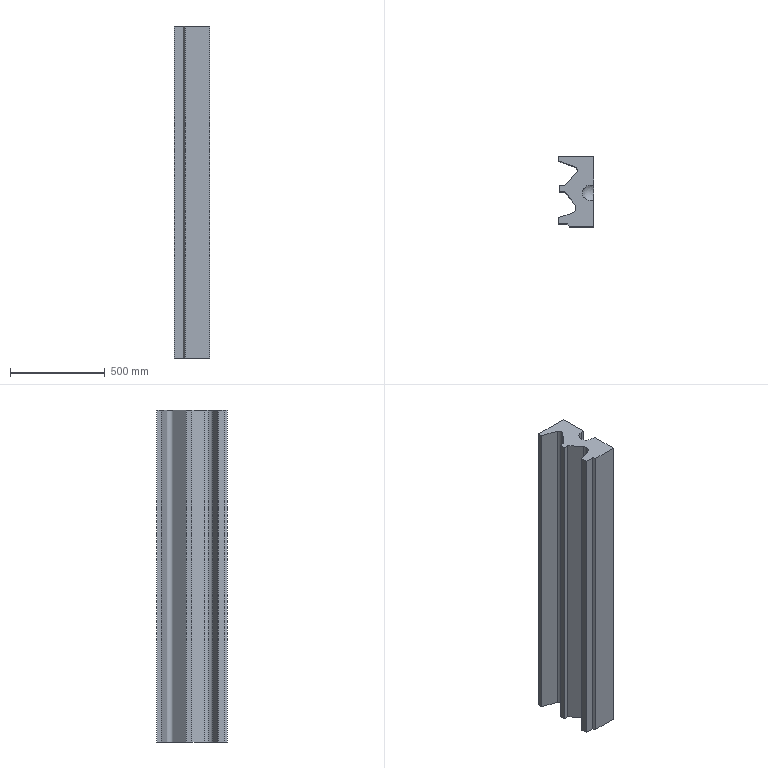Part | SolidWorks | features 3DProfileFeature 1, Extrusion 1, ICE 1, MirrorPattern 1, RevCut 1 | 1 solid | 33 faces | box 187.997 x 370.453 x 1750 mm | volume 86925596 mm3 | plane 24 | cylinder 5 | spline 2 | sphere 2 | commonest cylinder face diameters 80 x3 63.152 x2
STEP:
#1=CARTESIAN_POINT('',(-20.,75.362,-1650.));
#2=VERTEX_POINT('',#1);
#3=CARTESIAN_POINT('',(-60.,35.362,-1650.));
#4=VERTEX_POINT('',#3);
#5=CARTESIAN_POINT('',(-20.,35.362,-1650.));
#6=DIRECTION('',(0.,0.,1.));
#7=DIRECTION('',(-1.,0.,0.));
#8=AXIS2_PLACEMENT_3D('',#5,#6,#7);
#9=CIRCLE('',#8,40.);
#10=EDGE_CURVE('',#2,#4,#9,.T.);
#11=ORIENTED_EDGE('',*,*,#10,.T.);
#12=CARTESIAN_POINT('',(-60.,35.362,-1750.));
#13=VERTEX_POINT('',#12);
#14=CARTESIAN_POINT('',(-60.,35.362,-1650.));
#15=DIRECTION('',(0.,0.,-1.));
#16=VECTOR('',#15,1000.);
#17=LINE('',#14,#16);
#18=EDGE_CURVE('',#4,#13,#17,.T.);
#19=ORIENTED_EDGE('',*,*,#18,.T.);
#20=CARTESIAN_POINT('',(-20.,75.362,-1750.));
#21=VERTEX_POINT('',#20);
#22=CARTESIAN_POINT('',(-20.,35.362,-1750.));
#23=DIRECTION('',(0.,0.,1.));
#24=DIRECTION('',(-1.,0.,0.));
#25=AXIS2_PLACEMENT_3D('',#22,#23,#24);
#26=CIRCLE('',#25,40.);
#27=EDGE_CURVE('',#21,#13,#26,.T.);
#28=ORIENTED_EDGE('',*,*,#27,.F.);
#29=CARTESIAN_POINT('',(-20.,75.362,-1650.));
#30=DIRECTION('',(0.,0.,-1.));
#31=VECTOR('',#30,1000.);
#32=LINE('',#29,#31);
#33=EDGE_CURVE('',#2,#21,#32,.T.);
#34=ORIENTED_EDGE('',*,*,#33,.F.);
#35=EDGE_LOOP('',(#11,#19,#28,#34));
#36=FACE_OUTER_BOUND('',#35,.T.);
#37=CARTESIAN_POINT('',(-20.,35.362,-1650.));
#38=DIRECTION('',(0.,0.,-1.));
#39=DIRECTION('',(-1.,0.,0.));
#40=AXIS2_PLACEMENT_3D('',#37,#38,#39);
#41=CYLINDRICAL_SURFACE('',#40,40.);
#42=ADVANCED_FACE('',(#36),#41,.F.);
#43=CARTESIAN_POINT('',(-95.739,-44.185,-1750.));
#44=VERTEX_POINT('',#43);
#45=CARTESIAN_POINT('',(-102.315,-24.897,-1750.));
#46=VERTEX_POINT('',#45);
#47=CARTESIAN_POINT('',(-127.315,-44.185,-1750.));
#48=DIRECTION('',(0.,0.,1.));
#49=DIRECTION('',(1.,0.,0.));
#50=AXIS2_PLACEMENT_3D('',#47,#48,#49);
#51=CIRCLE('',#50,31.576);
#52=EDGE_CURVE('',#44,#46,#51,.T.);
#53=ORIENTED_EDGE('',*,*,#52,.F.);
#54=CARTESIAN_POINT('',(-95.739,-44.185,0.));
#55=VERTEX_POINT('',#54);
#56=CARTESIAN_POINT('',(-95.739,-44.185,-1750.));
#57=DIRECTION('',(0.,0.,1.));
#58=VECTOR('',#57,1000.);
#59=LINE('',#56,#58);
#60=EDGE_CURVE('',#44,#55,#59,.T.);
#61=ORIENTED_EDGE('',*,*,#60,.T.);
#62=CARTESIAN_POINT('',(-102.315,-24.897,0.));
#63=VERTEX_POINT('',#62);
#64=CARTESIAN_POINT('',(-127.315,-44.185,0.));
#65=DIRECTION('',(0.,0.,1.));
#66=DIRECTION('',(1.,0.,0.));
#67=AXIS2_PLACEMENT_3D('',#64,#65,#66);
#68=CIRCLE('',#67,31.576);
#69=EDGE_CURVE('',#55,#63,#68,.T.);
#70=ORIENTED_EDGE('',*,*,#69,.T.);
#71=CARTESIAN_POINT('',(-102.315,-24.897,-1750.));
#72=DIRECTION('',(0.,0.,1.));
#73=VECTOR('',#72,1000.);
#74=LINE('',#71,#73);
#75=EDGE_CURVE('',#46,#63,#74,.T.);
#76=ORIENTED_EDGE('',*,*,#75,.F.);
#77=EDGE_LOOP('',(#53,#61,#70,#76));
#78=FACE_OUTER_BOUND('',#77,.T.);
#79=CARTESIAN_POINT('',(-127.315,-44.185,-1750.));
#80=DIRECTION('',(0.,0.,1.));
#81=DIRECTION('',(1.,0.,0.));
#82=AXIS2_PLACEMENT_3D('',#79,#80,#81);
#83=CYLINDRICAL_SURFACE('',#82,31.576);
#84=ADVANCED_FACE('',(#78),#83,.F.);
#85=CARTESIAN_POINT('',(0.,-4.638,-1650.));
#86=VERTEX_POINT('',#85);
#87=CARTESIAN_POINT('',(0.,-24.638,-1650.));
#88=VERTEX_POINT('',#87);
#89=CARTESIAN_POINT('',(0.,95.362,-1650.));
#90=DIRECTION('',(0.,-1.,0.));
#91=VECTOR('',#90,1000.);
#92=LINE('',#89,#91);
#93=EDGE_CURVE('',#86,#88,#92,.T.);
#94=ORIENTED_EDGE('',*,*,#93,.T.);
#95=CARTESIAN_POINT('',(0.,95.362,-1650.));
#96=VERTEX_POINT('',#95);
#97=CARTESIAN_POINT('',(0.,35.362,-1650.));
#98=DIRECTION('',(-1.,0.,0.));
#99=DIRECTION('',(0.,-1.,0.));
#100=AXIS2_PLACEMENT_3D('',#97,#98,#99);
#101=CIRCLE('',#100,60.);
#102=EDGE_CURVE('',#88,#96,#101,.T.);
#103=ORIENTED_EDGE('',*,*,#102,.T.);
#104=CARTESIAN_POINT('',(0.,75.362,-1650.));
#105=VERTEX_POINT('',#104);
#106=CARTESIAN_POINT('',(0.,95.362,-1650.));
#107=DIRECTION('',(0.,-1.,0.));
#108=VECTOR('',#107,1000.);
#109=LINE('',#106,#108);
#110=EDGE_CURVE('',#96,#105,#109,.T.);
#111=ORIENTED_EDGE('',*,*,#110,.T.);
#112=CARTESIAN_POINT('',(0.,75.362,-1750.));
#113=VERTEX_POINT('',#112);
#114=CARTESIAN_POINT('',(0.,75.362,-1650.));
#115=DIRECTION('',(0.,0.,-1.));
#116=VECTOR('',#115,1000.);
#117=LINE('',#114,#116);
#118=EDGE_CURVE('',#105,#113,#117,.T.);
#119=ORIENTED_EDGE('',*,*,#118,.T.);
#120=CARTESIAN_POINT('',(0.,225.815,-1750.));
#121=VERTEX_POINT('',#120);
#122=CARTESIAN_POINT('',(0.,0.,-1750.));
#123=DIRECTION('',(0.,1.,0.));
#124=VECTOR('',#123,1000.);
#125=LINE('',#122,#124);
#126=EDGE_CURVE('',#113,#121,#125,.T.);
#127=ORIENTED_EDGE('',*,*,#126,.T.);
#128=CARTESIAN_POINT('',(0.,225.815,0.));
#129=VERTEX_POINT('',#128);
#130=CARTESIAN_POINT('',(0.,225.815,-1750.));
#131=DIRECTION('',(0.,0.,1.));
#132=VECTOR('',#131,1000.);
#133=LINE('',#130,#132);
#134=EDGE_CURVE('',#121,#129,#133,.T.);
#135=ORIENTED_EDGE('',*,*,#134,.T.);
#136=CARTESIAN_POINT('',(0.,75.362,0.));
#137=VERTEX_POINT('',#136);
#138=CARTESIAN_POINT('',(0.,0.,0.));
#139=DIRECTION('',(0.,1.,0.));
#140=VECTOR('',#139,1000.);
#141=LINE('',#138,#140);
#142=EDGE_CURVE('',#137,#129,#141,.T.);
#143=ORIENTED_EDGE('',*,*,#142,.F.);
#144=CARTESIAN_POINT('',(0.,75.362,-100.));
#145=VERTEX_POINT('',#144);
#146=CARTESIAN_POINT('',(0.,75.362,-100.));
#147=DIRECTION('',(0.,0.,1.));
#148=VECTOR('',#147,1000.);
#149=LINE('',#146,#148);
#150=EDGE_CURVE('',#145,#137,#149,.T.);
#151=ORIENTED_EDGE('',*,*,#150,.F.);
#152=CARTESIAN_POINT('',(0.,95.362,-100.));
#153=VERTEX_POINT('',#152);
#154=CARTESIAN_POINT('',(0.,95.362,-100.));
#155=DIRECTION('',(0.,-1.,0.));
#156=VECTOR('',#155,1000.);
#157=LINE('',#154,#156);
#158=EDGE_CURVE('',#153,#145,#157,.T.);
#159=ORIENTED_EDGE('',*,*,#158,.F.);
#160=CARTESIAN_POINT('',(0.,-24.638,-100.));
#161=VERTEX_POINT('',#160);
#162=CARTESIAN_POINT('',(0.,35.362,-100.));
#163=DIRECTION('',(1.,0.,0.));
#164=DIRECTION('',(0.,-1.,0.));
#165=AXIS2_PLACEMENT_3D('',#162,#163,#164);
#166=CIRCLE('',#165,60.);
#167=EDGE_CURVE('',#161,#153,#166,.T.);
#168=ORIENTED_EDGE('',*,*,#167,.F.);
#169=CARTESIAN_POINT('',(0.,-4.638,-100.));
#170=VERTEX_POINT('',#169);
#171=CARTESIAN_POINT('',(0.,95.362,-100.));
#172=DIRECTION('',(0.,-1.,0.));
#173=VECTOR('',#172,1000.);
#174=LINE('',#171,#173);
#175=EDGE_CURVE('',#170,#161,#174,.T.);
#176=ORIENTED_EDGE('',*,*,#175,.F.);
#177=CARTESIAN_POINT('',(0.,-4.638,0.));
#178=VERTEX_POINT('',#177);
#179=CARTESIAN_POINT('',(0.,-4.638,-100.));
#180=DIRECTION('',(0.,0.,1.));
#181=VECTOR('',#180,1000.);
#182=LINE('',#179,#181);
#183=EDGE_CURVE('',#170,#178,#182,.T.);
#184=ORIENTED_EDGE('',*,*,#183,.T.);
#185=CARTESIAN_POINT('',(0.,-144.638,0.));
#186=VERTEX_POINT('',#185);
#187=CARTESIAN_POINT('',(0.,0.,0.));
#188=DIRECTION('',(0.,1.,0.));
#189=VECTOR('',#188,1000.);
#190=LINE('',#187,#189);
#191=EDGE_CURVE('',#186,#178,#190,.T.);
#192=ORIENTED_EDGE('',*,*,#191,.F.);
#193=CARTESIAN_POINT('',(0.,-144.638,-1750.));
#194=VERTEX_POINT('',#193);
#195=CARTESIAN_POINT('',(0.,-144.638,-1750.));
#196=DIRECTION('',(0.,0.,1.));
#197=VECTOR('',#196,1000.);
#198=LINE('',#195,#197);
#199=EDGE_CURVE('',#194,#186,#198,.T.);
#200=ORIENTED_EDGE('',*,*,#199,.F.);
#201=CARTESIAN_POINT('',(0.,-4.638,-1750.));
#202=VERTEX_POINT('',#201);
#203=CARTESIAN_POINT('',(0.,0.,-1750.));
#204=DIRECTION('',(0.,1.,0.));
#205=VECTOR('',#204,1000.);
#206=LINE('',#203,#205);
#207=EDGE_CURVE('',#194,#202,#206,.T.);
#208=ORIENTED_EDGE('',*,*,#207,.T.);
#209=CARTESIAN_POINT('',(0.,-4.638,-1650.));
#210=DIRECTION('',(0.,0.,-1.));
#211=VECTOR('',#210,1000.);
#212=LINE('',#209,#211);
#213=EDGE_CURVE('',#86,#202,#212,.T.);
#214=ORIENTED_EDGE('',*,*,#213,.F.);
#215=EDGE_LOOP('',(#94,#103,#111,#119,#127,#135,#143,#151,#159,#168,#176,#184,#192,#200,#208,#214));
#216=FACE_OUTER_BOUND('',#215,.T.);
#217=CARTESIAN_POINT('',(0.,0.,-1750.));
#218=DIRECTION('',(1.,0.,0.));
#219=DIRECTION('',(0.,0.,-1.));
#220=AXIS2_PLACEMENT_3D('',#217,#218,#219);
#221=PLANE('',#220);
#222=ADVANCED_FACE('',(#216),#221,.T.);
#223=CARTESIAN_POINT('',(-20.,75.362,-1750.));
#224=DIRECTION('',(-1.,0.,0.));
#225=VECTOR('',#224,1000.);
#226=LINE('',#223,#225);
#227=EDGE_CURVE('',#113,#21,#226,.T.);
#228=ORIENTED_EDGE('',*,*,#227,.T.);
#229=ORIENTED_EDGE('',*,*,#27,.T.);
#230=CARTESIAN_POINT('',(-20.,-4.638,-1750.));
#231=VERTEX_POINT('',#230);
#232=CARTESIAN_POINT('',(-20.,35.362,-1750.));
#233=DIRECTION('',(0.,0.,1.));
#234=DIRECTION('',(-1.,0.,0.));
#235=AXIS2_PLACEMENT_3D('',#232,#233,#234);
#236=CIRCLE('',#235,40.);
#237=EDGE_CURVE('',#13,#231,#236,.T.);
#238=ORIENTED_EDGE('',*,*,#237,.T.);
#239=CARTESIAN_POINT('',(0.,-4.638,-1750.));
#240=DIRECTION('',(1.,0.,0.));
#241=VECTOR('',#240,1000.);
#242=LINE('',#239,#241);
#243=EDGE_CURVE('',#231,#202,#242,.T.);
#244=ORIENTED_EDGE('',*,*,#243,.T.);
#245=ORIENTED_EDGE('',*,*,#207,.F.);
#246=CARTESIAN_POINT('',(-130.,-144.638,-1750.));
#247=VERTEX_POINT('',#246);
#248=CARTESIAN_POINT('',(0.,-144.638,-1750.));
#249=DIRECTION('',(-1.,0.,0.));
#250=VECTOR('',#249,1000.);
#251=LINE('',#248,#250);
#252=EDGE_CURVE('',#194,#247,#251,.T.);
#253=ORIENTED_EDGE('',*,*,#252,.T.);
#254=CARTESIAN_POINT('',(-140.3,-129.189,-1750.));
#255=VERTEX_POINT('',#254);
#256=CARTESIAN_POINT('',(-156.756,-104.504,-1750.));
#257=DIRECTION('',(-0.5547,0.8321,0.));
#258=VECTOR('',#257,1000.);
#259=LINE('',#256,#258);
#260=EDGE_CURVE('',#247,#255,#259,.T.);
#261=ORIENTED_EDGE('',*,*,#260,.T.);
#262=CARTESIAN_POINT('',(-187.997,-129.189,-1750.));
#263=VERTEX_POINT('',#262);
#264=CARTESIAN_POINT('',(0.,-129.189,-1750.));
#265=DIRECTION('',(-1.,0.,0.));
#266=VECTOR('',#265,1000.);
#267=LINE('',#264,#266);
#268=EDGE_CURVE('',#255,#263,#267,.T.);
#269=ORIENTED_EDGE('',*,*,#268,.T.);
#270=CARTESIAN_POINT('',(-187.997,-99.189,-1750.));
#271=VERTEX_POINT('',#270);
#272=CARTESIAN_POINT('',(-187.997,0.,-1750.));
#273=DIRECTION('',(0.,1.,0.));
#274=VECTOR('',#273,1000.);
#275=LINE('',#272,#274);
#276=EDGE_CURVE('',#263,#271,#275,.T.);
#277=ORIENTED_EDGE('',*,*,#276,.T.);
#278=CARTESIAN_POINT('',(-185.804,-96.424,-1750.));
#279=VERTEX_POINT('',#278);
#280=CARTESIAN_POINT('',(-187.997,-99.189,-1750.));
#281=CARTESIAN_POINT('',(-187.738,-97.242,-1750.));
#282=CARTESIAN_POINT('',(-185.804,-96.424,-1750.));
#283=B_SPLINE_CURVE_WITH_KNOTS('',2,(#280,#281,#282),.UNSPECIFIED.,.F.,.F.,(3,3),(0.,1.),.UNSPECIFIED.);
#284=EDGE_CURVE('',#271,#279,#283,.T.);
#285=ORIENTED_EDGE('',*,*,#284,.T.);
#286=CARTESIAN_POINT('',(-108.027,-69.185,-1750.));
#287=VERTEX_POINT('',#286);
#288=CARTESIAN_POINT('',(9.78,-27.927,-1750.));
#289=DIRECTION('',(0.9438,0.3305,0.));
#290=VECTOR('',#289,1000.);
#291=LINE('',#288,#290);
#292=EDGE_CURVE('',#279,#287,#291,.T.);
#293=ORIENTED_EDGE('',*,*,#292,.T.);
#294=CARTESIAN_POINT('',(-127.315,-44.185,-1750.));
#295=DIRECTION('',(0.,0.,1.));
#296=DIRECTION('',(1.,0.,0.));
#297=AXIS2_PLACEMENT_3D('',#294,#295,#296);
#298=CIRCLE('',#297,31.576);
#299=EDGE_CURVE('',#287,#44,#298,.T.);
#300=ORIENTED_EDGE('',*,*,#299,.T.);
#301=ORIENTED_EDGE('',*,*,#52,.T.);
#302=CARTESIAN_POINT('',(-153.014,40.815,-1750.));
#303=VERTEX_POINT('',#302);
#304=CARTESIAN_POINT('',(-76.178,-58.774,-1750.));
#305=DIRECTION('',(-0.6109,0.7917,0.));
#306=VECTOR('',#305,1000.);
#307=LINE('',#304,#306);
#308=EDGE_CURVE('',#46,#303,#307,.T.);
#309=ORIENTED_EDGE('',*,*,#308,.T.);
#310=CARTESIAN_POINT('',(-180.014,40.815,-1750.));
#311=VERTEX_POINT('',#310);
#312=CARTESIAN_POINT('',(0.,40.815,-1750.));
#313=DIRECTION('',(-1.,0.,0.));
#314=VECTOR('',#313,1000.);
#315=LINE('',#312,#314);
#316=EDGE_CURVE('',#303,#311,#315,.T.);
#317=ORIENTED_EDGE('',*,*,#316,.T.);
#318=CARTESIAN_POINT('',(-180.014,70.815,-1750.));
#319=VERTEX_POINT('',#318);
#320=CARTESIAN_POINT('',(-180.014,0.,-1750.));
#321=DIRECTION('',(0.,1.,0.));
#322=VECTOR('',#321,1000.);
#323=LINE('',#320,#322);
#324=EDGE_CURVE('',#311,#319,#323,.T.);
#325=ORIENTED_EDGE('',*,*,#324,.T.);
#326=CARTESIAN_POINT('',(-153.014,70.815,-1750.));
#327=VERTEX_POINT('',#326);
#328=CARTESIAN_POINT('',(0.,70.815,-1750.));
#329=DIRECTION('',(1.,0.,0.));
#330=VECTOR('',#329,1000.);
#331=LINE('',#328,#330);
#332=EDGE_CURVE('',#319,#327,#331,.T.);
#333=ORIENTED_EDGE('',*,*,#332,.T.);
#334=CARTESIAN_POINT('',(-92.192,140.123,-1750.));
#335=VERTEX_POINT('',#334);
#336=CARTESIAN_POINT('',(-121.551,106.668,-1750.));
#337=DIRECTION('',(-0.6596,-0.7516,0.));
#338=VECTOR('',#337,1000.);
#339=LINE('',#336,#338);
#340=EDGE_CURVE('',#335,#327,#339,.T.);
#341=ORIENTED_EDGE('',*,*,#340,.F.);
#342=CARTESIAN_POINT('',(-100.014,173.289,-1750.));
#343=VERTEX_POINT('',#342);
#344=CARTESIAN_POINT('',(-100.014,173.289,-1750.));
#345=CARTESIAN_POINT('',(-89.242,167.173,-1750.));
#346=CARTESIAN_POINT('',(-82.492,150.195,-1750.));
#347=CARTESIAN_POINT('',(-92.192,140.123,-1750.));
#348=B_SPLINE_CURVE_WITH_KNOTS('',3,(#344,#345,#346,#347),.UNSPECIFIED.,.F.,.F.,(4,4),(0.,1.),.UNSPECIFIED.);
#349=EDGE_CURVE('',#343,#335,#348,.T.);
#350=ORIENTED_EDGE('',*,*,#349,.F.);
#351=CARTESIAN_POINT('',(-185.804,202.815,-1750.));
#352=VERTEX_POINT('',#351);
#353=CARTESIAN_POINT('',(42.732,124.162,-1750.));
#354=DIRECTION('',(0.9456,-0.3254,0.));
#355=VECTOR('',#354,1000.);
#356=LINE('',#353,#355);
#357=EDGE_CURVE('',#352,#343,#356,.T.);
#358=ORIENTED_EDGE('',*,*,#357,.F.);
#359=CARTESIAN_POINT('',(-185.804,225.815,-1750.));
#360=VERTEX_POINT('',#359);
#361=CARTESIAN_POINT('',(-185.804,0.,-1750.));
#362=DIRECTION('',(0.,-1.,0.));
#363=VECTOR('',#362,1000.);
#364=LINE('',#361,#363);
#365=EDGE_CURVE('',#360,#352,#364,.T.);
#366=ORIENTED_EDGE('',*,*,#365,.F.);
#367=CARTESIAN_POINT('',(0.,225.815,-1750.));
#368=DIRECTION('',(-1.,0.,0.));
#369=VECTOR('',#368,1000.);
#370=LINE('',#367,#369);
#371=EDGE_CURVE('',#121,#360,#370,.T.);
#372=ORIENTED_EDGE('',*,*,#371,.F.);
#373=ORIENTED_EDGE('',*,*,#126,.F.);
#374=EDGE_LOOP('',(#228,#229,#238,#244,#245,#253,#261,#269,#277,#285,#293,#300,#301,#309,#317,#325,#333,#341,#350,#358,#366,#372,#373));
#375=FACE_OUTER_BOUND('',#374,.T.);
#376=CARTESIAN_POINT('',(0.,0.,-1750.));
#377=DIRECTION('',(0.,0.,1.));
#378=DIRECTION('',(1.,0.,0.));
#379=AXIS2_PLACEMENT_3D('',#376,#377,#378);
#380=PLANE('',#379);
#381=ADVANCED_FACE('',(#375),#380,.F.);
#382=CARTESIAN_POINT('',(-185.804,202.815,0.));
#383=VERTEX_POINT('',#382);
#384=CARTESIAN_POINT('',(-100.014,173.289,0.));
#385=VERTEX_POINT('',#384);
#386=CARTESIAN_POINT('',(42.732,124.162,0.));
#387=DIRECTION('',(0.9456,-0.3254,0.));
#388=VECTOR('',#387,1000.);
#389=LINE('',#386,#388);
#390=EDGE_CURVE('',#383,#385,#389,.T.);
#391=ORIENTED_EDGE('',*,*,#390,.F.);
#392=CARTESIAN_POINT('',(-185.804,202.815,-1750.));
#393=DIRECTION('',(0.,0.,1.));
#394=VECTOR('',#393,1000.);
#395=LINE('',#392,#394);
#396=EDGE_CURVE('',#352,#383,#395,.T.);
#397=ORIENTED_EDGE('',*,*,#396,.F.);
#398=ORIENTED_EDGE('',*,*,#357,.T.);
#399=CARTESIAN_POINT('',(-100.014,173.289,-1750.));
#400=DIRECTION('',(0.,0.,1.));
#401=VECTOR('',#400,1000.);
#402=LINE('',#399,#401);
#403=EDGE_CURVE('',#343,#385,#402,.T.);
#404=ORIENTED_EDGE('',*,*,#403,.T.);
#405=EDGE_LOOP('',(#391,#397,#398,#404));
#406=FACE_OUTER_BOUND('',#405,.T.);
#407=CARTESIAN_POINT('',(42.732,124.162,-1750.));
#408=DIRECTION('',(-0.3254,-0.9456,0.));
#409=DIRECTION('',(0.9456,-0.3254,0.));
#410=AXIS2_PLACEMENT_3D('',#407,#408,#409);
#411=PLANE('',#410);
#412=ADVANCED_FACE('',(#406),#411,.T.);
#413=CARTESIAN_POINT('',(-185.804,225.815,0.));
#414=VERTEX_POINT('',#413);
#415=CARTESIAN_POINT('',(-185.804,0.,0.));
#416=DIRECTION('',(0.,-1.,0.));
#417=VECTOR('',#416,1000.);
#418=LINE('',#415,#417);
#419=EDGE_CURVE('',#414,#383,#418,.T.);
#420=ORIENTED_EDGE('',*,*,#419,.F.);
#421=CARTESIAN_POINT('',(-185.804,225.815,-1750.));
#422=DIRECTION('',(0.,0.,1.));
#423=VECTOR('',#422,1000.);
#424=LINE('',#421,#423);
#425=EDGE_CURVE('',#360,#414,#424,.T.);
#426=ORIENTED_EDGE('',*,*,#425,.F.);
#427=ORIENTED_EDGE('',*,*,#365,.T.);
#428=ORIENTED_EDGE('',*,*,#396,.T.);
#429=EDGE_LOOP('',(#420,#426,#427,#428));
#430=FACE_OUTER_BOUND('',#429,.T.);
#431=CARTESIAN_POINT('',(-185.804,0.,-1750.));
#432=DIRECTION('',(-1.,0.,0.));
#433=DIRECTION('',(0.,0.,1.));
#434=AXIS2_PLACEMENT_3D('',#431,#432,#433);
#435=PLANE('',#434);
#436=ADVANCED_FACE('',(#430),#435,.T.);
#437=CARTESIAN_POINT('',(0.,225.815,0.));
#438=DIRECTION('',(-1.,0.,0.));
#439=VECTOR('',#438,1000.);
#440=LINE('',#437,#439);
#441=EDGE_CURVE('',#129,#414,#440,.T.);
#442=ORIENTED_EDGE('',*,*,#441,.F.);
#443=ORIENTED_EDGE('',*,*,#134,.F.);
#444=ORIENTED_EDGE('',*,*,#371,.T.);
#445=ORIENTED_EDGE('',*,*,#425,.T.);
#446=EDGE_LOOP('',(#442,#443,#444,#445));
#447=FACE_OUTER_BOUND('',#446,.T.);
#448=CARTESIAN_POINT('',(0.,225.815,-1750.));
#449=DIRECTION('',(0.,1.,0.));
#450=DIRECTION('',(0.,0.,1.));
#451=AXIS2_PLACEMENT_3D('',#448,#449,#450);
#452=PLANE('',#451);
#453=ADVANCED_FACE('',(#447),#452,.T.);
#454=CARTESIAN_POINT('',(-130.,-144.638,0.));
#455=VERTEX_POINT('',#454);
#456=CARTESIAN_POINT('',(0.,-144.638,0.));
#457=DIRECTION('',(-1.,0.,0.));
#458=VECTOR('',#457,1000.);
#459=LINE('',#456,#458);
#460=EDGE_CURVE('',#186,#455,#459,.T.);
#461=ORIENTED_EDGE('',*,*,#460,.T.);
#462=CARTESIAN_POINT('',(-130.,-144.638,-1750.));
#463=DIRECTION('',(0.,0.,1.));
#464=VECTOR('',#463,1000.);
#465=LINE('',#462,#464);
#466=EDGE_CURVE('',#247,#455,#465,.T.);
#467=ORIENTED_EDGE('',*,*,#466,.F.);
#468=ORIENTED_EDGE('',*,*,#252,.F.);
#469=ORIENTED_EDGE('',*,*,#199,.T.);
#470=EDGE_LOOP('',(#461,#467,#468,#469));
#471=FACE_OUTER_BOUND('',#470,.T.);
#472=CARTESIAN_POINT('',(0.,-144.638,-1750.));
#473=DIRECTION('',(0.,1.,0.));
#474=DIRECTION('',(0.,0.,1.));
#475=AXIS2_PLACEMENT_3D('',#472,#473,#474);
#476=PLANE('',#475);
#477=ADVANCED_FACE('',(#471),#476,.F.);
#478=CARTESIAN_POINT('',(-140.3,-129.189,0.));
#479=VERTEX_POINT('',#478);
#480=CARTESIAN_POINT('',(-156.756,-104.504,0.));
#481=DIRECTION('',(-0.5547,0.8321,0.));
#482=VECTOR('',#481,1000.);
#483=LINE('',#480,#482);
#484=EDGE_CURVE('',#455,#479,#483,.T.);
#485=ORIENTED_EDGE('',*,*,#484,.T.);
#486=CARTESIAN_POINT('',(-140.3,-129.189,-1750.));
#487=DIRECTION('',(0.,0.,1.));
#488=VECTOR('',#487,1000.);
#489=LINE('',#486,#488);
#490=EDGE_CURVE('',#255,#479,#489,.T.);
#491=ORIENTED_EDGE('',*,*,#490,.F.);
#492=ORIENTED_EDGE('',*,*,#260,.F.);
#493=ORIENTED_EDGE('',*,*,#466,.T.);
#494=EDGE_LOOP('',(#485,#491,#492,#493));
#495=FACE_OUTER_BOUND('',#494,.T.);
#496=CARTESIAN_POINT('',(-156.756,-104.504,-1750.));
#497=DIRECTION('',(0.8321,0.5547,0.));
#498=DIRECTION('',(-0.5547,0.8321,0.));
#499=AXIS2_PLACEMENT_3D('',#496,#497,#498);
#500=PLANE('',#499);
#501=ADVANCED_FACE('',(#495),#500,.F.);
#502=CARTESIAN_POINT('',(-187.997,-129.189,0.));
#503=VERTEX_POINT('',#502);
#504=CARTESIAN_POINT('',(0.,-129.189,0.));
#505=DIRECTION('',(-1.,0.,0.));
#506=VECTOR('',#505,1000.);
#507=LINE('',#504,#506);
#508=EDGE_CURVE('',#479,#503,#507,.T.);
#509=ORIENTED_EDGE('',*,*,#508,.T.);
#510=CARTESIAN_POINT('',(-187.997,-129.189,-1750.));
#511=DIRECTION('',(0.,0.,1.));
#512=VECTOR('',#511,1000.);
#513=LINE('',#510,#512);
#514=EDGE_CURVE('',#263,#503,#513,.T.);
#515=ORIENTED_EDGE('',*,*,#514,.F.);
#516=ORIENTED_EDGE('',*,*,#268,.F.);
#517=ORIENTED_EDGE('',*,*,#490,.T.);
#518=EDGE_LOOP('',(#509,#515,#516,#517));
#519=FACE_OUTER_BOUND('',#518,.T.);
#520=CARTESIAN_POINT('',(0.,-129.189,-1750.));
#521=DIRECTION('',(0.,1.,0.));
#522=DIRECTION('',(-1.,0.,0.));
#523=AXIS2_PLACEMENT_3D('',#520,#521,#522);
#524=PLANE('',#523);
#525=ADVANCED_FACE('',(#519),#524,.F.);
#526=CARTESIAN_POINT('',(-187.997,-99.189,0.));
#527=VERTEX_POINT('',#526);
#528=CARTESIAN_POINT('',(-187.997,0.,0.));
#529=DIRECTION('',(0.,1.,0.));
#530=VECTOR('',#529,1000.);
#531=LINE('',#528,#530);
#532=EDGE_CURVE('',#503,#527,#531,.T.);
#533=ORIENTED_EDGE('',*,*,#532,.T.);
#534=CARTESIAN_POINT('',(-187.997,-99.189,-1750.));
#535=DIRECTION('',(0.,0.,1.));
#536=VECTOR('',#535,1000.);
#537=LINE('',#534,#536);
#538=EDGE_CURVE('',#271,#527,#537,.T.);
#539=ORIENTED_EDGE('',*,*,#538,.F.);
#540=ORIENTED_EDGE('',*,*,#276,.F.);
#541=ORIENTED_EDGE('',*,*,#514,.T.);
#542=EDGE_LOOP('',(#533,#539,#540,#541));
#543=FACE_OUTER_BOUND('',#542,.T.);
#544=CARTESIAN_POINT('',(-187.997,0.,-1750.));
#545=DIRECTION('',(1.,0.,0.));
#546=DIRECTION('',(0.,0.,-1.));
#547=AXIS2_PLACEMENT_3D('',#544,#545,#546);
#548=PLANE('',#547);
#549=ADVANCED_FACE('',(#543),#548,.F.);
#550=CARTESIAN_POINT('',(-185.804,-96.424,0.));
#551=VERTEX_POINT('',#550);
#552=CARTESIAN_POINT('',(-187.997,-99.189,0.));
#553=CARTESIAN_POINT('',(-187.738,-97.242,0.));
#554=CARTESIAN_POINT('',(-185.804,-96.424,0.));
#555=B_SPLINE_CURVE_WITH_KNOTS('',2,(#552,#553,#554),.UNSPECIFIED.,.F.,.F.,(3,3),(0.,1.),.UNSPECIFIED.);
#556=EDGE_CURVE('',#527,#551,#555,.T.);
#557=ORIENTED_EDGE('',*,*,#556,.T.);
#558=CARTESIAN_POINT('',(-185.804,-96.424,-1750.));
#559=DIRECTION('',(0.,0.,1.));
#560=VECTOR('',#559,1000.);
#561=LINE('',#558,#560);
#562=EDGE_CURVE('',#279,#551,#561,.T.);
#563=ORIENTED_EDGE('',*,*,#562,.F.);
#564=ORIENTED_EDGE('',*,*,#284,.F.);
#565=ORIENTED_EDGE('',*,*,#538,.T.);
#566=EDGE_LOOP('',(#557,#563,#564,#565));
#567=FACE_OUTER_BOUND('',#566,.T.);
#568=CARTESIAN_POINT('',(-187.997,-99.189,-1750.));
#569=CARTESIAN_POINT('',(-187.997,-99.189,0.));
#570=CARTESIAN_POINT('',(-187.738,-97.242,-1750.));
#571=CARTESIAN_POINT('',(-187.738,-97.242,0.));
#572=CARTESIAN_POINT('',(-185.804,-96.424,-1750.));
#573=CARTESIAN_POINT('',(-185.804,-96.424,0.));
#574=B_SPLINE_SURFACE_WITH_KNOTS('',2,1,((#568,#569),(#570,#571),(#572,#573)),.UNSPECIFIED.,.F.,.F.,.F.,(3,3),(2,2),(0.,1.),(0.,1.),.UNSPECIFIED.);
#575=ADVANCED_FACE('',(#567),#574,.F.);
#576=CARTESIAN_POINT('',(-108.027,-69.185,0.));
#577=VERTEX_POINT('',#576);
#578=CARTESIAN_POINT('',(9.78,-27.927,0.));
#579=DIRECTION('',(0.9438,0.3305,0.));
#580=VECTOR('',#579,1000.);
#581=LINE('',#578,#580);
#582=EDGE_CURVE('',#551,#577,#581,.T.);
#583=ORIENTED_EDGE('',*,*,#582,.T.);
#584=CARTESIAN_POINT('',(-108.027,-69.185,-1750.));
#585=DIRECTION('',(0.,0.,1.));
#586=VECTOR('',#585,1000.);
#587=LINE('',#584,#586);
#588=EDGE_CURVE('',#287,#577,#587,.T.);
#589=ORIENTED_EDGE('',*,*,#588,.F.);
#590=ORIENTED_EDGE('',*,*,#292,.F.);
#591=ORIENTED_EDGE('',*,*,#562,.T.);
#592=EDGE_LOOP('',(#583,#589,#590,#591));
#593=FACE_OUTER_BOUND('',#592,.T.);
#594=CARTESIAN_POINT('',(9.78,-27.927,-1750.));
#595=DIRECTION('',(0.3305,-0.9438,0.));
#596=DIRECTION('',(0.9438,0.3305,0.));
#597=AXIS2_PLACEMENT_3D('',#594,#595,#596);
#598=PLANE('',#597);
#599=ADVANCED_FACE('',(#593),#598,.F.);
#600=ORIENTED_EDGE('',*,*,#60,.F.);
#601=ORIENTED_EDGE('',*,*,#299,.F.);
#602=ORIENTED_EDGE('',*,*,#588,.T.);
#603=CARTESIAN_POINT('',(-127.315,-44.185,0.));
#604=DIRECTION('',(0.,0.,1.));
#605=DIRECTION('',(1.,0.,0.));
#606=AXIS2_PLACEMENT_3D('',#603,#604,#605);
#607=CIRCLE('',#606,31.576);
#608=EDGE_CURVE('',#577,#55,#607,.T.);
#609=ORIENTED_EDGE('',*,*,#608,.T.);
#610=EDGE_LOOP('',(#600,#601,#602,#609));
#611=FACE_OUTER_BOUND('',#610,.T.);
#612=CARTESIAN_POINT('',(-127.315,-44.185,-1750.));
#613=DIRECTION('',(0.,0.,1.));
#614=DIRECTION('',(1.,0.,0.));
#615=AXIS2_PLACEMENT_3D('',#612,#613,#614);
#616=CYLINDRICAL_SURFACE('',#615,31.576);
#617=ADVANCED_FACE('',(#611),#616,.F.);
#618=CARTESIAN_POINT('',(-153.014,40.815,0.));
#619=VERTEX_POINT('',#618);
#620=CARTESIAN_POINT('',(-76.178,-58.774,0.));
#621=DIRECTION('',(-0.6109,0.7917,0.));
#622=VECTOR('',#621,1000.);
#623=LINE('',#620,#622);
#624=EDGE_CURVE('',#63,#619,#623,.T.);
#625=ORIENTED_EDGE('',*,*,#624,.T.);
#626=CARTESIAN_POINT('',(-153.014,40.815,-1750.));
#627=DIRECTION('',(0.,0.,1.));
#628=VECTOR('',#627,1000.);
#629=LINE('',#626,#628);
#630=EDGE_CURVE('',#303,#619,#629,.T.);
#631=ORIENTED_EDGE('',*,*,#630,.F.);
#632=ORIENTED_EDGE('',*,*,#308,.F.);
#633=ORIENTED_EDGE('',*,*,#75,.T.);
#634=EDGE_LOOP('',(#625,#631,#632,#633));
#635=FACE_OUTER_BOUND('',#634,.T.);
#636=CARTESIAN_POINT('',(-76.178,-58.774,-1750.));
#637=DIRECTION('',(0.7917,0.6109,0.));
#638=DIRECTION('',(-0.6109,0.7917,0.));
#639=AXIS2_PLACEMENT_3D('',#636,#637,#638);
#640=PLANE('',#639);
#641=ADVANCED_FACE('',(#635),#640,.F.);
#642=CARTESIAN_POINT('',(-180.014,40.815,0.));
#643=VERTEX_POINT('',#642);
#644=CARTESIAN_POINT('',(0.,40.815,0.));
#645=DIRECTION('',(-1.,0.,0.));
#646=VECTOR('',#645,1000.);
#647=LINE('',#644,#646);
#648=EDGE_CURVE('',#619,#643,#647,.T.);
#649=ORIENTED_EDGE('',*,*,#648,.T.);
#650=CARTESIAN_POINT('',(-180.014,40.815,-1750.));
#651=DIRECTION('',(0.,0.,1.));
#652=VECTOR('',#651,1000.);
#653=LINE('',#650,#652);
#654=EDGE_CURVE('',#311,#643,#653,.T.);
#655=ORIENTED_EDGE('',*,*,#654,.F.);
#656=ORIENTED_EDGE('',*,*,#316,.F.);
#657=ORIENTED_EDGE('',*,*,#630,.T.);
#658=EDGE_LOOP('',(#649,#655,#656,#657));
#659=FACE_OUTER_BOUND('',#658,.T.);
#660=CARTESIAN_POINT('',(0.,40.815,-1750.));
#661=DIRECTION('',(0.,1.,0.));
#662=DIRECTION('',(0.,0.,1.));
#663=AXIS2_PLACEMENT_3D('',#660,#661,#662);
#664=PLANE('',#663);
#665=ADVANCED_FACE('',(#659),#664,.F.);
#666=CARTESIAN_POINT('',(-180.014,70.815,0.));
#667=VERTEX_POINT('',#666);
#668=CARTESIAN_POINT('',(-180.014,0.,0.));
#669=DIRECTION('',(0.,1.,0.));
#670=VECTOR('',#669,1000.);
#671=LINE('',#668,#670);
#672=EDGE_CURVE('',#643,#667,#671,.T.);
#673=ORIENTED_EDGE('',*,*,#672,.T.);
#674=CARTESIAN_POINT('',(-180.014,70.815,-1750.));
#675=DIRECTION('',(0.,0.,1.));
#676=VECTOR('',#675,1000.);
#677=LINE('',#674,#676);
#678=EDGE_CURVE('',#319,#667,#677,.T.);
#679=ORIENTED_EDGE('',*,*,#678,.F.);
#680=ORIENTED_EDGE('',*,*,#324,.F.);
#681=ORIENTED_EDGE('',*,*,#654,.T.);
#682=EDGE_LOOP('',(#673,#679,#680,#681));
#683=FACE_OUTER_BOUND('',#682,.T.);
#684=CARTESIAN_POINT('',(-180.014,0.,-1750.));
#685=DIRECTION('',(1.,0.,0.));
#686=DIRECTION('',(0.,0.,-1.));
#687=AXIS2_PLACEMENT_3D('',#684,#685,#686);
#688=PLANE('',#687);
#689=ADVANCED_FACE('',(#683),#688,.F.);
#690=CARTESIAN_POINT('',(-153.014,70.815,0.));
#691=VERTEX_POINT('',#690);
#692=CARTESIAN_POINT('',(0.,70.815,0.));
#693=DIRECTION('',(1.,0.,0.));
#694=VECTOR('',#693,1000.);
#695=LINE('',#692,#694);
#696=EDGE_CURVE('',#667,#691,#695,.T.);
#697=ORIENTED_EDGE('',*,*,#696,.T.);
#698=CARTESIAN_POINT('',(-153.014,70.815,-1750.));
#699=DIRECTION('',(0.,0.,1.));
#700=VECTOR('',#699,1000.);
#701=LINE('',#698,#700);
#702=EDGE_CURVE('',#327,#691,#701,.T.);
#703=ORIENTED_EDGE('',*,*,#702,.F.);
#704=ORIENTED_EDGE('',*,*,#332,.F.);
#705=ORIENTED_EDGE('',*,*,#678,.T.);
#706=EDGE_LOOP('',(#697,#703,#704,#705));
#707=FACE_OUTER_BOUND('',#706,.T.);
#708=CARTESIAN_POINT('',(0.,70.815,-1750.));
#709=DIRECTION('',(0.,-1.,0.));
#710=DIRECTION('',(0.,0.,-1.));
#711=AXIS2_PLACEMENT_3D('',#708,#709,#710);
#712=PLANE('',#711);
#713=ADVANCED_FACE('',(#707),#712,.F.);
#714=CARTESIAN_POINT('',(-92.192,140.123,0.));
#715=VERTEX_POINT('',#714);
#716=CARTESIAN_POINT('',(-121.551,106.668,0.));
#717=DIRECTION('',(-0.6596,-0.7516,0.));
#718=VECTOR('',#717,1000.);
#719=LINE('',#716,#718);
#720=EDGE_CURVE('',#715,#691,#719,.T.);
#721=ORIENTED_EDGE('',*,*,#720,.F.);
#722=CARTESIAN_POINT('',(-92.192,140.123,-1750.));
#723=DIRECTION('',(0.,0.,1.));
#724=VECTOR('',#723,1000.);
#725=LINE('',#722,#724);
#726=EDGE_CURVE('',#335,#715,#725,.T.);
#727=ORIENTED_EDGE('',*,*,#726,.F.);
#728=ORIENTED_EDGE('',*,*,#340,.T.);
#729=ORIENTED_EDGE('',*,*,#702,.T.);
#730=EDGE_LOOP('',(#721,#727,#728,#729));
#731=FACE_OUTER_BOUND('',#730,.T.);
#732=CARTESIAN_POINT('',(-121.551,106.668,-1750.));
#733=DIRECTION('',(-0.7516,0.6596,0.));
#734=DIRECTION('',(-0.6596,-0.7516,0.));
#735=AXIS2_PLACEMENT_3D('',#732,#733,#734);
#736=PLANE('',#735);
#737=ADVANCED_FACE('',(#731),#736,.T.);
#738=CARTESIAN_POINT('',(-100.014,173.289,0.));
#739=CARTESIAN_POINT('',(-89.242,167.173,0.));
#740=CARTESIAN_POINT('',(-82.492,150.195,0.));
#741=CARTESIAN_POINT('',(-92.192,140.123,0.));
#742=B_SPLINE_CURVE_WITH_KNOTS('',3,(#738,#739,#740,#741),.UNSPECIFIED.,.F.,.F.,(4,4),(0.,1.),.UNSPECIFIED.);
#743=EDGE_CURVE('',#385,#715,#742,.T.);
#744=ORIENTED_EDGE('',*,*,#743,.F.);
#745=ORIENTED_EDGE('',*,*,#403,.F.);
#746=ORIENTED_EDGE('',*,*,#349,.T.);
#747=ORIENTED_EDGE('',*,*,#726,.T.);
#748=EDGE_LOOP('',(#744,#745,#746,#747));
#749=FACE_OUTER_BOUND('',#748,.T.);
#750=CARTESIAN_POINT('',(-100.014,173.289,-1750.));
#751=CARTESIAN_POINT('',(-100.014,173.289,0.));
#752=CARTESIAN_POINT('',(-89.242,167.173,-1750.));
#753=CARTESIAN_POINT('',(-89.242,167.173,0.));
#754=CARTESIAN_POINT('',(-82.492,150.195,-1750.));
#755=CARTESIAN_POINT('',(-82.492,150.195,0.));
#756=CARTESIAN_POINT('',(-92.192,140.123,-1750.));
#757=CARTESIAN_POINT('',(-92.192,140.123,0.));
#758=B_SPLINE_SURFACE_WITH_KNOTS('',3,1,((#750,#751),(#752,#753),(#754,#755),(#756,#757)),.UNSPECIFIED.,.F.,.F.,.F.,(4,4),(2,2),(0.,1.),(0.,1.),.UNSPECIFIED.);
#759=ADVANCED_FACE('',(#749),#758,.T.);
#760=CARTESIAN_POINT('',(-20.,-4.638,0.));
#761=VERTEX_POINT('',#760);
#762=CARTESIAN_POINT('',(0.,-4.638,0.));
#763=DIRECTION('',(1.,0.,0.));
#764=VECTOR('',#763,1000.);
#765=LINE('',#762,#764);
#766=EDGE_CURVE('',#761,#178,#765,.T.);
#767=ORIENTED_EDGE('',*,*,#766,.F.);
#768=CARTESIAN_POINT('',(-20.,75.362,0.));
#769=VERTEX_POINT('',#768);
#770=CARTESIAN_POINT('',(-20.,35.362,0.));
#771=DIRECTION('',(0.,0.,1.));
#772=DIRECTION('',(-1.,0.,0.));
#773=AXIS2_PLACEMENT_3D('',#770,#771,#772);
#774=CIRCLE('',#773,40.);
#775=EDGE_CURVE('',#769,#761,#774,.T.);
#776=ORIENTED_EDGE('',*,*,#775,.F.);
#777=CARTESIAN_POINT('',(-20.,75.362,0.));
#778=DIRECTION('',(-1.,0.,0.));
#779=VECTOR('',#778,1000.);
#780=LINE('',#777,#779);
#781=EDGE_CURVE('',#137,#769,#780,.T.);
#782=ORIENTED_EDGE('',*,*,#781,.F.);
#783=ORIENTED_EDGE('',*,*,#142,.T.);
#784=ORIENTED_EDGE('',*,*,#441,.T.);
#785=ORIENTED_EDGE('',*,*,#419,.T.);
#786=ORIENTED_EDGE('',*,*,#390,.T.);
#787=ORIENTED_EDGE('',*,*,#743,.T.);
#788=ORIENTED_EDGE('',*,*,#720,.T.);
#789=ORIENTED_EDGE('',*,*,#696,.F.);
#790=ORIENTED_EDGE('',*,*,#672,.F.);
#791=ORIENTED_EDGE('',*,*,#648,.F.);
#792=ORIENTED_EDGE('',*,*,#624,.F.);
#793=ORIENTED_EDGE('',*,*,#69,.F.);
#794=ORIENTED_EDGE('',*,*,#608,.F.);
#795=ORIENTED_EDGE('',*,*,#582,.F.);
#796=ORIENTED_EDGE('',*,*,#556,.F.);
#797=ORIENTED_EDGE('',*,*,#532,.F.);
#798=ORIENTED_EDGE('',*,*,#508,.F.);
#799=ORIENTED_EDGE('',*,*,#484,.F.);
#800=ORIENTED_EDGE('',*,*,#460,.F.);
#801=ORIENTED_EDGE('',*,*,#191,.T.);
#802=EDGE_LOOP('',(#767,#776,#782,#783,#784,#785,#786,#787,#788,#789,#790,#791,#792,#793,#794,#795,#796,#797,#798,#799,#800,#801));
#803=FACE_OUTER_BOUND('',#802,.T.);
#804=CARTESIAN_POINT('',(0.,0.,0.));
#805=DIRECTION('',(0.,0.,1.));
#806=DIRECTION('',(1.,0.,0.));
#807=AXIS2_PLACEMENT_3D('',#804,#805,#806);
#808=PLANE('',#807);
#809=ADVANCED_FACE('',(#803),#808,.T.);
#810=ORIENTED_EDGE('',*,*,#766,.T.);
#811=ORIENTED_EDGE('',*,*,#183,.F.);
#812=CARTESIAN_POINT('',(-20.,-4.638,-100.));
#813=VERTEX_POINT('',#812);
#814=CARTESIAN_POINT('',(0.,-4.638,-100.));
#815=DIRECTION('',(1.,0.,0.));
#816=VECTOR('',#815,1000.);
#817=LINE('',#814,#816);
#818=EDGE_CURVE('',#813,#170,#817,.T.);
#819=ORIENTED_EDGE('',*,*,#818,.F.);
#820=CARTESIAN_POINT('',(-20.,-4.638,-100.));
#821=DIRECTION('',(0.,0.,1.));
#822=VECTOR('',#821,1000.);
#823=LINE('',#820,#822);
#824=EDGE_CURVE('',#813,#761,#823,.T.);
#825=ORIENTED_EDGE('',*,*,#824,.T.);
#826=EDGE_LOOP('',(#810,#811,#819,#825));
#827=FACE_OUTER_BOUND('',#826,.T.);
#828=CARTESIAN_POINT('',(0.,-4.638,-100.));
#829=DIRECTION('',(0.,-1.,0.));
#830=DIRECTION('',(1.,0.,0.));
#831=AXIS2_PLACEMENT_3D('',#828,#829,#830);
#832=PLANE('',#831);
#833=ADVANCED_FACE('',(#827),#832,.F.);
#834=ORIENTED_EDGE('',*,*,#775,.T.);
#835=ORIENTED_EDGE('',*,*,#824,.F.);
#836=CARTESIAN_POINT('',(-60.,35.362,-100.));
#837=VERTEX_POINT('',#836);
#838=CARTESIAN_POINT('',(-20.,35.362,-100.));
#839=DIRECTION('',(0.,0.,1.));
#840=DIRECTION('',(-1.,0.,0.));
#841=AXIS2_PLACEMENT_3D('',#838,#839,#840);
#842=CIRCLE('',#841,40.);
#843=EDGE_CURVE('',#837,#813,#842,.T.);
#844=ORIENTED_EDGE('',*,*,#843,.F.);
#845=CARTESIAN_POINT('',(-20.,75.362,-100.));
#846=VERTEX_POINT('',#845);
#847=CARTESIAN_POINT('',(-20.,35.362,-100.));
#848=DIRECTION('',(0.,0.,1.));
#849=DIRECTION('',(-1.,0.,0.));
#850=AXIS2_PLACEMENT_3D('',#847,#848,#849);
#851=CIRCLE('',#850,40.);
#852=EDGE_CURVE('',#846,#837,#851,.T.);
#853=ORIENTED_EDGE('',*,*,#852,.F.);
#854=CARTESIAN_POINT('',(-20.,75.362,-100.));
#855=DIRECTION('',(0.,0.,1.));
#856=VECTOR('',#855,1000.);
#857=LINE('',#854,#856);
#858=EDGE_CURVE('',#846,#769,#857,.T.);
#859=ORIENTED_EDGE('',*,*,#858,.T.);
#860=EDGE_LOOP('',(#834,#835,#844,#853,#859));
#861=FACE_OUTER_BOUND('',#860,.T.);
#862=CARTESIAN_POINT('',(-20.,35.362,-100.));
#863=DIRECTION('',(0.,0.,1.));
#864=DIRECTION('',(1.,0.,0.));
#865=AXIS2_PLACEMENT_3D('',#862,#863,#864);
#866=CYLINDRICAL_SURFACE('',#865,40.);
#867=ADVANCED_FACE('',(#861),#866,.F.);
#868=ORIENTED_EDGE('',*,*,#781,.T.);
#869=ORIENTED_EDGE('',*,*,#858,.F.);
#870=CARTESIAN_POINT('',(-20.,75.362,-100.));
#871=DIRECTION('',(-1.,0.,0.));
#872=VECTOR('',#871,1000.);
#873=LINE('',#870,#872);
#874=EDGE_CURVE('',#145,#846,#873,.T.);
#875=ORIENTED_EDGE('',*,*,#874,.F.);
#876=ORIENTED_EDGE('',*,*,#150,.T.);
#877=EDGE_LOOP('',(#868,#869,#875,#876));
#878=FACE_OUTER_BOUND('',#877,.T.);
#879=CARTESIAN_POINT('',(-20.,75.362,-100.));
#880=DIRECTION('',(0.,1.,0.));
#881=DIRECTION('',(0.,0.,1.));
#882=AXIS2_PLACEMENT_3D('',#879,#880,#881);
#883=PLANE('',#882);
#884=ADVANCED_FACE('',(#878),#883,.F.);
#885=ORIENTED_EDGE('',*,*,#175,.T.);
#886=CARTESIAN_POINT('',(0.,35.362,-100.));
#887=DIRECTION('',(0.,0.,-1.));
#888=DIRECTION('',(0.,-1.,0.));
#889=AXIS2_PLACEMENT_3D('',#886,#887,#888);
#890=CIRCLE('',#889,60.);
#891=EDGE_CURVE('',#161,#837,#890,.T.);
#892=ORIENTED_EDGE('',*,*,#891,.T.);
#893=ORIENTED_EDGE('',*,*,#843,.T.);
#894=ORIENTED_EDGE('',*,*,#818,.T.);
#895=EDGE_LOOP('',(#885,#892,#893,#894));
#896=FACE_OUTER_BOUND('',#895,.T.);
#897=CARTESIAN_POINT('',(0.,35.362,-100.));
#898=DIRECTION('',(0.,0.,1.));
#899=DIRECTION('',(0.,-1.,0.));
#900=AXIS2_PLACEMENT_3D('',#897,#898,#899);
#901=PLANE('',#900);
#902=ADVANCED_FACE('',(#896),#901,.F.);
#903=CARTESIAN_POINT('',(0.,35.362,-100.));
#904=DIRECTION('',(0.,0.,-1.));
#905=DIRECTION('',(0.,-1.,0.));
#906=AXIS2_PLACEMENT_3D('',#903,#904,#905);
#907=CIRCLE('',#906,60.);
#908=EDGE_CURVE('',#837,#153,#907,.T.);
#909=ORIENTED_EDGE('',*,*,#908,.T.);
#910=ORIENTED_EDGE('',*,*,#158,.T.);
#911=ORIENTED_EDGE('',*,*,#874,.T.);
#912=ORIENTED_EDGE('',*,*,#852,.T.);
#913=EDGE_LOOP('',(#909,#910,#911,#912));
#914=FACE_OUTER_BOUND('',#913,.T.);
#915=CARTESIAN_POINT('',(0.,35.362,-100.));
#916=DIRECTION('',(0.,0.,1.));
#917=DIRECTION('',(0.,-1.,0.));
#918=AXIS2_PLACEMENT_3D('',#915,#916,#917);
#919=PLANE('',#918);
#920=ADVANCED_FACE('',(#914),#919,.F.);
#921=ORIENTED_EDGE('',*,*,#167,.T.);
#922=ORIENTED_EDGE('',*,*,#908,.F.);
#923=ORIENTED_EDGE('',*,*,#891,.F.);
#924=EDGE_LOOP('',(#921,#922,#923));
#925=FACE_OUTER_BOUND('',#924,.T.);
#926=CARTESIAN_POINT('',(0.,35.362,-100.));
#927=DIRECTION('',(0.,0.,-1.));
#928=DIRECTION('',(-1.,0.,0.));
#929=AXIS2_PLACEMENT_3D('',#926,#927,#928);
#930=SPHERICAL_SURFACE('',#929,60.);
#931=ADVANCED_FACE('',(#925),#930,.F.);
#932=ORIENTED_EDGE('',*,*,#227,.F.);
#933=ORIENTED_EDGE('',*,*,#118,.F.);
#934=CARTESIAN_POINT('',(-20.,75.362,-1650.));
#935=DIRECTION('',(-1.,0.,0.));
#936=VECTOR('',#935,1000.);
#937=LINE('',#934,#936);
#938=EDGE_CURVE('',#105,#2,#937,.T.);
#939=ORIENTED_EDGE('',*,*,#938,.T.);
#940=ORIENTED_EDGE('',*,*,#33,.T.);
#941=EDGE_LOOP('',(#932,#933,#939,#940));
#942=FACE_OUTER_BOUND('',#941,.T.);
#943=CARTESIAN_POINT('',(-20.,75.362,-1650.));
#944=DIRECTION('',(0.,-1.,0.));
#945=DIRECTION('',(0.,0.,-1.));
#946=AXIS2_PLACEMENT_3D('',#943,#944,#945);
#947=PLANE('',#946);
#948=ADVANCED_FACE('',(#942),#947,.T.);
#949=ORIENTED_EDGE('',*,*,#18,.F.);
#950=CARTESIAN_POINT('',(-20.,-4.638,-1650.));
#951=VERTEX_POINT('',#950);
#952=CARTESIAN_POINT('',(-20.,35.362,-1650.));
#953=DIRECTION('',(0.,0.,1.));
#954=DIRECTION('',(-1.,0.,0.));
#955=AXIS2_PLACEMENT_3D('',#952,#953,#954);
#956=CIRCLE('',#955,40.);
#957=EDGE_CURVE('',#4,#951,#956,.T.);
#958=ORIENTED_EDGE('',*,*,#957,.T.);
#959=CARTESIAN_POINT('',(-20.,-4.638,-1650.));
#960=DIRECTION('',(0.,0.,-1.));
#961=VECTOR('',#960,1000.);
#962=LINE('',#959,#961);
#963=EDGE_CURVE('',#951,#231,#962,.T.);
#964=ORIENTED_EDGE('',*,*,#963,.T.);
#965=ORIENTED_EDGE('',*,*,#237,.F.);
#966=EDGE_LOOP('',(#949,#958,#964,#965));
#967=FACE_OUTER_BOUND('',#966,.T.);
#968=CARTESIAN_POINT('',(-20.,35.362,-1650.));
#969=DIRECTION('',(0.,0.,-1.));
#970=DIRECTION('',(-1.,0.,0.));
#971=AXIS2_PLACEMENT_3D('',#968,#969,#970);
#972=CYLINDRICAL_SURFACE('',#971,40.);
#973=ADVANCED_FACE('',(#967),#972,.F.);
#974=ORIENTED_EDGE('',*,*,#243,.F.);
#975=ORIENTED_EDGE('',*,*,#963,.F.);
#976=CARTESIAN_POINT('',(0.,-4.638,-1650.));
#977=DIRECTION('',(1.,0.,0.));
#978=VECTOR('',#977,1000.);
#979=LINE('',#976,#978);
#980=EDGE_CURVE('',#951,#86,#979,.T.);
#981=ORIENTED_EDGE('',*,*,#980,.T.);
#982=ORIENTED_EDGE('',*,*,#213,.T.);
#983=EDGE_LOOP('',(#974,#975,#981,#982));
#984=FACE_OUTER_BOUND('',#983,.T.);
#985=CARTESIAN_POINT('',(0.,-4.638,-1650.));
#986=DIRECTION('',(0.,1.,0.));
#987=DIRECTION('',(-1.,0.,0.));
#988=AXIS2_PLACEMENT_3D('',#985,#986,#987);
#989=PLANE('',#988);
#990=ADVANCED_FACE('',(#984),#989,.T.);
#991=ORIENTED_EDGE('',*,*,#938,.F.);
#992=ORIENTED_EDGE('',*,*,#110,.F.);
#993=CARTESIAN_POINT('',(0.,35.362,-1650.));
#994=DIRECTION('',(0.,0.,-1.));
#995=DIRECTION('',(0.,-1.,0.));
#996=AXIS2_PLACEMENT_3D('',#993,#994,#995);
#997=CIRCLE('',#996,60.);
#998=EDGE_CURVE('',#4,#96,#997,.T.);
#999=ORIENTED_EDGE('',*,*,#998,.F.);
#1000=ORIENTED_EDGE('',*,*,#10,.F.);
#1001=EDGE_LOOP('',(#991,#992,#999,#1000));
#1002=FACE_OUTER_BOUND('',#1001,.T.);
#1003=CARTESIAN_POINT('',(0.,35.362,-1650.));
#1004=DIRECTION('',(0.,0.,-1.));
#1005=DIRECTION('',(0.,-1.,0.));
#1006=AXIS2_PLACEMENT_3D('',#1003,#1004,#1005);
#1007=PLANE('',#1006);
#1008=ADVANCED_FACE('',(#1002),#1007,.F.);
#1009=ORIENTED_EDGE('',*,*,#102,.F.);
#1010=CARTESIAN_POINT('',(0.,35.362,-1650.));
#1011=DIRECTION('',(0.,0.,-1.));
#1012=DIRECTION('',(0.,-1.,0.));
#1013=AXIS2_PLACEMENT_3D('',#1010,#1011,#1012);
#1014=CIRCLE('',#1013,60.);
#1015=EDGE_CURVE('',#88,#4,#1014,.T.);
#1016=ORIENTED_EDGE('',*,*,#1015,.T.);
#1017=ORIENTED_EDGE('',*,*,#998,.T.);
#1018=EDGE_LOOP('',(#1009,#1016,#1017));
#1019=FACE_OUTER_BOUND('',#1018,.T.);
#1020=CARTESIAN_POINT('',(0.,35.362,-1650.));
#1021=DIRECTION('',(0.,0.,-1.));
#1022=DIRECTION('',(-1.,0.,0.));
#1023=AXIS2_PLACEMENT_3D('',#1020,#1021,#1022);
#1024=SPHERICAL_SURFACE('',#1023,60.);
#1025=ADVANCED_FACE('',(#1019),#1024,.F.);
#1026=ORIENTED_EDGE('',*,*,#957,.F.);
#1027=ORIENTED_EDGE('',*,*,#1015,.F.);
#1028=ORIENTED_EDGE('',*,*,#93,.F.);
#1029=ORIENTED_EDGE('',*,*,#980,.F.);
#1030=EDGE_LOOP('',(#1026,#1027,#1028,#1029));
#1031=FACE_OUTER_BOUND('',#1030,.T.);
#1032=CARTESIAN_POINT('',(0.,35.362,-1650.));
#1033=DIRECTION('',(0.,0.,-1.));
#1034=DIRECTION('',(0.,-1.,0.));
#1035=AXIS2_PLACEMENT_3D('',#1032,#1033,#1034);
#1036=PLANE('',#1035);
#1037=ADVANCED_FACE('',(#1031),#1036,.F.);
#1038=CLOSED_SHELL('',(#42,#84,#222,#381,#412,#436,#453,#477,#501,#525,#549,#575,#599,#617,#641,#665,#689,#713,#737,#759,#809,#833,#867,#884,#902,#920,#931,#948,#973,#990,#1008,#1025,#1037));
#1039=MANIFOLD_SOLID_BREP('',#1038);
#1040=CARTESIAN_POINT('',(0.,0.,0.));
#1041=DIRECTION('',(0.,0.,1.));
#1042=DIRECTION('',(1.,0.,0.));
#1043=AXIS2_PLACEMENT_3D('',#1040,#1041,#1042);
#1044=(LENGTH_UNIT()NAMED_UNIT(*)SI_UNIT(.MILLI.,.METRE.));
#1045=UNCERTAINTY_MEASURE_WITH_UNIT(LENGTH_MEASURE(0.00001),#1044,'','');
#1046=(NAMED_UNIT(*)PLANE_ANGLE_UNIT()SI_UNIT($,.RADIAN.));
#1047=(NAMED_UNIT(*)SI_UNIT($,.STERADIAN.)SOLID_ANGLE_UNIT());
#1048=(GEOMETRIC_REPRESENTATION_CONTEXT(3)GLOBAL_UNCERTAINTY_ASSIGNED_CONTEXT((#1045))GLOBAL_UNIT_ASSIGNED_CONTEXT((#1044,#1046,#1047))REPRESENTATION_CONTEXT('',''));
#1049=ADVANCED_BREP_SHAPE_REPRESENTATION('',(#1039,#1043),#1048);